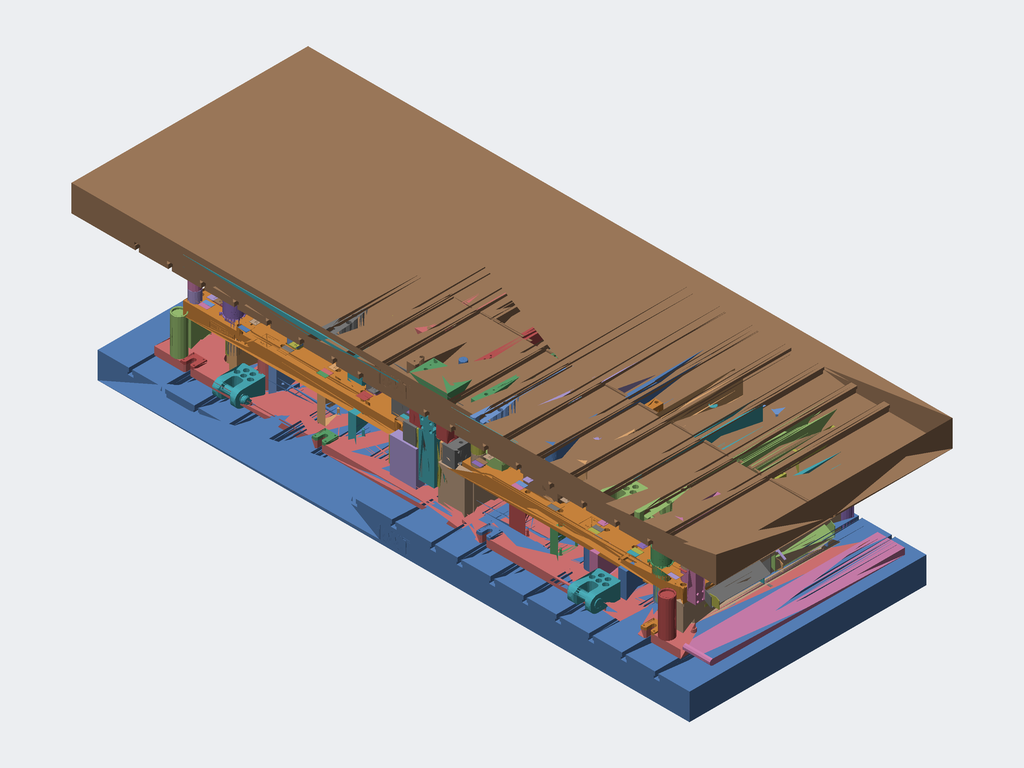Assembly | STEP file | 1269 different items | 1269 placed
Parts list (item | name | quantity | parent item | size | volume), first 346 of 1269 items:
1 | 008_id4090_x_t | x1 | in lll_x_t | 80 x 80 x 85 mm | 404567 mm3
2 | 008_id4094_x_t | x1 | in lll_x_t | 80 x 80 x 85 mm | 404567 mm3
3 | 008_id4098_x_t | x1 | in lll_x_t | 80 x 80 x 85 mm | 404567 mm3
4 | 008_id4122_x_t | x1 | in lll_x_t | 80 x 80 x 85 mm | 404311 mm3
5 | 008_id4126_x_t | x1 | in lll_x_t | 80 x 80 x 85 mm | 404567 mm3
6 | 008_id4130_x_t | x1 | in lll_x_t | 80 x 80 x 85 mm | 404311 mm3
7 | 014_id2546_x_t | x1 | in lll_x_t | 80 x 80 x 137.5 mm | 639951 mm3
8 | 014_id2550_x_t | x1 | in lll_x_t | 80 x 80 x 137.5 mm | 639951 mm3
9 | 014_id2554_x_t | x1 | in lll_x_t | 80 x 80 x 137.5 mm | 639951 mm3
10 | 014_id2558_x_t | x1 | in lll_x_t | 80 x 80 x 137.5 mm | 639951 mm3
11 | 014_id2562_x_t | x1 | in lll_x_t | 80 x 80 x 137.5 mm | 639951 mm3
12 | 014_id2842_x_t | x1 | in lll_x_t | 80 x 80 x 137.5 mm | 639951 mm3
13 | 103_id3510_x_t | x1 | in lll_x_t | 115 x 32.999 x 20 mm | 61100 mm3
14 | 180_id4502_x_t | x1 | in lll_x_t | 235 x 230 x 80 mm | 2542104 mm3
15 | 180_id4582_x_t | x1 | in lll_x_t | 565 x 500 x 35 mm | 7605579 mm3
16 | 1_id1746_x_t | x1 | in lll_x_t | 36 x 36 x 216 mm | 99455 mm3
17 | 1_id1750_x_t | x1 | in lll_x_t | 36 x 36 x 216 mm | 99455 mm3
18 | 1_id1758_x_t | x1 | in lll_x_t | 36 x 36 x 216 mm | 99455 mm3
19 | 1_id1798_x_t | x1 | in lll_x_t | 18 x 18 x 52 mm | 7011 mm3
20 | 1_id1802_x_t | x1 | in lll_x_t | 18 x 18 x 52 mm | 7011 mm3
21 | 1_id1806_x_t | x1 | in lll_x_t | 18 x 18 x 52 mm | 7011 mm3
22 | 1_id1814_x_t | x1 | in lll_x_t | 18 x 18 x 52 mm | 7011 mm3
23 | 1_id1822_x_t | x1 | in lll_x_t | 18 x 18 x 52 mm | 7011 mm3
24 | 1_id1826_x_t | x1 | in lll_x_t | 18 x 18 x 52 mm | 7011 mm3
25 | 1_id1834_x_t | x1 | in lll_x_t | 18 x 18 x 52 mm | 7011 mm3
26 | 1_id1846_x_t | x1 | in lll_x_t | 18 x 18 x 52 mm | 7011 mm3
27 | 1_id1850_x_t | x1 | in lll_x_t | 18 x 18 x 52 mm | 7011 mm3
28 | 1_id1862_x_t | x1 | in lll_x_t | 18 x 18 x 52 mm | 7011 mm3
29 | 1_id1866_x_t | x1 | in lll_x_t | 18 x 18 x 52 mm | 7011 mm3
30 | 1_id1870_x_t | x1 | in lll_x_t | 18 x 18 x 52 mm | 7011 mm3
31 | 1_id1882_x_t | x1 | in lll_x_t | 18 x 18 x 52 mm | 7011 mm3
32 | 1_id1886_x_t | x1 | in lll_x_t | 18 x 18 x 52 mm | 7011 mm3
33 | 1_id1890_x_t | x1 | in lll_x_t | 18 x 18 x 52 mm | 7011 mm3
34 | 1_id1894_x_t | x1 | in lll_x_t | 18 x 18 x 52 mm | 7011 mm3
35 | 1_id1898_x_t | x1 | in lll_x_t | 18 x 18 x 52 mm | 7011 mm3
36 | 1_id1902_x_t | x1 | in lll_x_t | 18 x 18 x 52 mm | 7011 mm3
37 | 1_id1910_x_t | x1 | in lll_x_t | 18 x 18 x 52 mm | 7011 mm3
38 | 1_id1914_x_t | x1 | in lll_x_t | 18 x 18 x 52 mm | 7011 mm3
39 | 1_id1922_x_t | x1 | in lll_x_t | 18 x 18 x 52 mm | 7011 mm3
40 | 1_id1930_x_t | x1 | in lll_x_t | 18 x 18 x 52 mm | 7011 mm3
41 | 1_id1934_x_t | x1 | in lll_x_t | 18 x 18 x 52 mm | 7011 mm3
42 | 1_id1942_x_t | x1 | in lll_x_t | 18 x 18 x 52 mm | 7011 mm3
43 | 1_id1950_x_t | x1 | in lll_x_t | 18 x 18 x 52 mm | 7011 mm3
44 | 1_id1954_x_t | x1 | in lll_x_t | 18 x 18 x 52 mm | 7011 mm3
45 | 1_id1962_x_t | x1 | in lll_x_t | 18 x 18 x 52 mm | 7011 mm3
46 | 1_id1970_x_t | x1 | in lll_x_t | 18 x 18 x 52 mm | 7011 mm3
47 | 1_id1974_x_t | x1 | in lll_x_t | 18 x 18 x 52 mm | 7011 mm3
48 | 1_id1982_x_t | x1 | in lll_x_t | 18 x 18 x 52 mm | 7011 mm3
49 | 1_id1990_x_t | x1 | in lll_x_t | 18 x 18 x 52 mm | 7011 mm3
50 | 1_id1994_x_t | x1 | in lll_x_t | 18 x 18 x 52 mm | 7011 mm3
51 | 1_id2002_x_t | x1 | in lll_x_t | 18 x 18 x 52 mm | 7011 mm3
52 | 1_id2010_x_t | x1 | in lll_x_t | 18 x 18 x 52 mm | 7011 mm3
53 | 1_id2014_x_t | x1 | in lll_x_t | 18 x 18 x 52 mm | 7011 mm3
54 | 1_id2022_x_t | x1 | in lll_x_t | 18 x 18 x 52 mm | 7011 mm3
55 | 1_id2030_x_t | x1 | in lll_x_t | 18 x 18 x 52 mm | 7011 mm3
56 | 1_id2034_x_t | x1 | in lll_x_t | 18 x 18 x 52 mm | 7011 mm3
57 | 1_id2042_x_t | x1 | in lll_x_t | 18 x 18 x 52 mm | 7011 mm3
58 | 1_id2050_x_t | x1 | in lll_x_t | 18 x 18 x 52 mm | 7011 mm3
59 | 1_id2054_x_t | x1 | in lll_x_t | 18 x 18 x 52 mm | 7011 mm3
60 | 1_id2062_x_t | x1 | in lll_x_t | 18 x 18 x 52 mm | 7011 mm3
61 | 1_id2066_x_t | x1 | in lll_x_t | 18 x 18 x 52 mm | 7011 mm3
62 | 1_id2070_x_t | x1 | in lll_x_t | 18 x 18 x 52 mm | 7011 mm3
63 | 1_id2074_x_t | x1 | in lll_x_t | 18 x 18 x 52 mm | 7011 mm3
64 | 1_id2086_x_t | x1 | in lll_x_t | 18 x 18 x 52 mm | 7011 mm3
65 | 1_id2090_x_t | x1 | in lll_x_t | 18 x 18 x 52 mm | 7011 mm3
66 | 1_id2094_x_t | x1 | in lll_x_t | 18 x 18 x 52 mm | 7011 mm3
67 | 1_id2114_x_t | x1 | in lll_x_t | 18 x 18 x 52 mm | 7011 mm3
68 | 1_id2118_x_t | x1 | in lll_x_t | 18 x 18 x 52 mm | 7011 mm3
69 | 1_id2122_x_t | x1 | in lll_x_t | 18 x 18 x 52 mm | 7011 mm3
70 | 1_id2126_x_t | x1 | in lll_x_t | 18 x 18 x 52 mm | 7011 mm3
71 | 1_id2130_x_t | x1 | in lll_x_t | 18 x 18 x 52 mm | 7011 mm3
72 | 1_id2134_x_t | x1 | in lll_x_t | 18 x 18 x 52 mm | 7011 mm3
73 | 1_id2138_x_t | x1 | in lll_x_t | 18 x 18 x 52 mm | 7011 mm3
74 | 1_id2142_x_t | x1 | in lll_x_t | 18 x 18 x 52 mm | 7011 mm3
75 | 1_id2310_x_t | x1 | in lll_x_t | 63.2 x 63.2 x 294 mm | 592651 mm3
76 | 1_id2330_x_t | x1 | in lll_x_t | 75.2 x 75.2 x 295 mm | 855529 mm3
77 | 1_id2338_x_t | x1 | in lll_x_t | 63.2 x 63.2 x 294 mm | 592651 mm3
78 | 1_id2346_x_t | x1 | in lll_x_t | 63.2 x 63.2 x 294 mm | 592651 mm3
79 | 1_id2358_x_t | x1 | in lll_x_t | 63.2 x 63.2 x 294 mm | 592651 mm3
80 | 1_id2362_x_t | x1 | in lll_x_t | 63.2 x 63.2 x 294 mm | 592651 mm3
81 | 1_id2366_x_t | x1 | in lll_x_t | 63.2 x 63.2 x 294 mm | 592651 mm3
82 | 1_id2370_x_t | x1 | in lll_x_t | 63.2 x 63.2 x 294 mm | 592651 mm3
83 | 1_id2374_x_t | x1 | in lll_x_t | 63.2 x 63.2 x 294 mm | 592651 mm3
84 | 1_id2378_x_t | x1 | in lll_x_t | 63.2 x 63.2 x 294 mm | 592651 mm3
85 | 1_id2382_x_t | x1 | in lll_x_t | 63.2 x 63.2 x 294 mm | 592651 mm3
86 | 1_id2386_x_t | x1 | in lll_x_t | 63.2 x 63.2 x 294 mm | 592651 mm3
87 | 1_id2390_x_t | x1 | in lll_x_t | 63.2 x 63.2 x 294 mm | 592651 mm3
88 | 1_id2394_x_t | x1 | in lll_x_t | 63.2 x 63.2 x 294 mm | 592651 mm3
89 | 1_id2398_x_t | x1 | in lll_x_t | 63.2 x 63.2 x 294 mm | 592651 mm3
90 | 1_id2402_x_t | x1 | in lll_x_t | 63.2 x 63.2 x 294 mm | 592651 mm3
91 | 1_id2406_x_t | x1 | in lll_x_t | 63.2 x 63.2 x 294 mm | 592651 mm3
92 | 1_id2410_x_t | x1 | in lll_x_t | 63.2 x 63.2 x 294 mm | 592651 mm3
93 | 1_id2414_x_t | x1 | in lll_x_t | 63.2 x 63.2 x 294 mm | 592651 mm3
94 | 1_id2418_x_t | x1 | in lll_x_t | 75.2 x 75.2 x 295 mm | 855529 mm3
95 | 1_id2422_x_t | x1 | in lll_x_t | 63.2 x 63.2 x 294 mm | 592651 mm3
96 | 1_id2426_x_t | x1 | in lll_x_t | 63.2 x 63.2 x 294 mm | 592651 mm3
97 | 1_id2430_x_t | x1 | in lll_x_t | 63.2 x 63.2 x 294 mm | 592651 mm3
98 | 1_id2434_x_t | x1 | in lll_x_t | 63.2 x 63.2 x 294 mm | 592651 mm3
99 | 1_id2438_x_t | x1 | in lll_x_t | 63.2 x 63.2 x 294 mm | 592651 mm3
100 | 1_id2442_x_t | x1 | in lll_x_t | 63.2 x 63.2 x 294 mm | 592651 mm3
101 | 1_id2446_x_t | x1 | in lll_x_t | 63.2 x 63.2 x 294 mm | 592651 mm3
102 | 1_id2450_x_t | x1 | in lll_x_t | 63.2 x 63.2 x 294 mm | 592651 mm3
103 | 1_id2454_x_t | x1 | in lll_x_t | 75.2 x 75.2 x 295 mm | 855529 mm3
104 | 1_id2458_x_t | x1 | in lll_x_t | 95.2 x 95.2 x 308 mm | 1486829 mm3
105 | 1_id2462_x_t | x1 | in lll_x_t | 95.2 x 95.2 x 308 mm | 1486829 mm3
106 | 1_id2482_x_t | x1 | in lll_x_t | 217 x 240 x 120 mm | 3421641 mm3
107 | 1_id2486_x_t | x1 | in lll_x_t | 217 x 240 x 120 mm | 3421641 mm3
108 | 1_id2518_x_t | x1 | in lll_x_t | 36 x 36 x 216 mm | 99455 mm3
109 | 1_id2522_x_t | x1 | in lll_x_t | 36 x 36 x 216 mm | 99455 mm3
110 | 1_id2526_x_t | x1 | in lll_x_t | 36 x 36 x 216 mm | 99455 mm3
111 | 1_id282_x_t | x1 | in lll_x_t | 21 x 21 x 118.2 mm | 17923 mm3
112 | 1_id286_x_t | x1 | in lll_x_t | 21 x 21 x 118.2 mm | 17923 mm3
113 | 1_id290_x_t | x1 | in lll_x_t | 43 x 39 x 118.2 mm | 84183 mm3
114 | 1_id294_x_t | x1 | in lll_x_t | 43 x 39 x 118.2 mm | 84183 mm3
115 | 1_id3518_x_t | x1 | in lll_x_t | 37 x 37 x 118.2 mm | 77419 mm3
116 | 1_id3530_x_t | x1 | in lll_x_t | 37 x 37 x 118.2 mm | 77419 mm3
117 | 1_id3546_x_t | x1 | in lll_x_t | 37 x 37 x 118.2 mm | 77419 mm3
118 | 1_id3566_x_t | x1 | in lll_x_t | 30 x 26 x 118.2 mm | 45235 mm3
119 | 1_id3570_x_t | x1 | in lll_x_t | 37 x 37 x 118.2 mm | 77419 mm3
120 | 1_id3590_x_t | x1 | in lll_x_t | 37 x 37 x 118.2 mm | 77419 mm3
121 | 1_id3618_x_t | x1 | in lll_x_t | 37 x 37 x 118.2 mm | 77419 mm3
122 | 1_id3630_x_t | x1 | in lll_x_t | 37 x 37 x 118.2 mm | 77419 mm3
123 | 1_id3642_x_t | x1 | in lll_x_t | 25 x 22.5 x 118.2 mm | 27347 mm3
124 | 1_id3650_x_t | x1 | in lll_x_t | 30 x 26 x 118.2 mm | 45235 mm3
125 | 1_id3662_x_t | x1 | in lll_x_t | 25 x 25 x 118.2 mm | 30521 mm3
126 | 1_id3670_x_t | x1 | in lll_x_t | 25 x 25 x 118.2 mm | 30521 mm3
127 | 1_id3686_x_t | x1 | in lll_x_t | 25 x 22.5 x 118.2 mm | 27347 mm3
128 | 1_id3690_x_t | x1 | in lll_x_t | 37 x 37 x 118.2 mm | 77419 mm3
129 | 1_id3750_x_t | x1 | in lll_x_t | 28 x 28 x 222 mm | 65272 mm3
130 | 1_id3758_x_t | x1 | in lll_x_t | 28 x 28 x 222 mm | 65272 mm3
131 | 1_id3922_x_t | x1 | in lll_x_t | 45.2 x 45.2 x 405 mm | 414792 mm3
132 | 1_id3926_x_t | x1 | in lll_x_t | 45.2 x 45.2 x 405 mm | 414792 mm3
133 | 1_id3930_x_t | x1 | in lll_x_t | 45.2 x 45.2 x 405 mm | 414792 mm3
134 | 1_id3934_x_t | x1 | in lll_x_t | 45.2 x 45.2 x 405 mm | 414792 mm3
135 | 1_id3938_x_t | x1 | in lll_x_t | 45.2 x 45.2 x 405 mm | 414792 mm3
136 | 1_id3942_x_t | x1 | in lll_x_t | 45.2 x 45.2 x 405 mm | 414792 mm3
137 | 1_id3946_x_t | x1 | in lll_x_t | 45.2 x 45.2 x 405 mm | 414792 mm3
138 | 1_id3950_x_t | x1 | in lll_x_t | 45.2 x 45.2 x 405 mm | 414792 mm3
139 | 1_id3954_x_t | x1 | in lll_x_t | 45.2 x 45.2 x 405 mm | 414792 mm3
140 | 1_id3958_x_t | x1 | in lll_x_t | 45.2 x 45.2 x 405 mm | 414792 mm3
141 | 1_id3962_x_t | x1 | in lll_x_t | 45.2 x 45.2 x 405 mm | 414792 mm3
142 | 1_id3966_x_t | x1 | in lll_x_t | 45.2 x 45.2 x 405 mm | 414792 mm3
143 | 1_id3970_x_t | x1 | in lll_x_t | 45.2 x 45.2 x 405 mm | 414792 mm3
144 | 1_id3974_x_t | x1 | in lll_x_t | 45.2 x 45.2 x 405 mm | 414792 mm3
145 | 1_id3978_x_t | x1 | in lll_x_t | 45.2 x 45.2 x 405 mm | 414792 mm3
146 | 1_id4158_x_t | x1 | in lll_x_t | 16 x 16 x 40 mm | 4057 mm3
147 | 1_id4170_x_t | x1 | in lll_x_t | 16 x 16 x 40 mm | 4057 mm3
148 | 1_id4174_x_t | x1 | in lll_x_t | 16 x 16 x 40 mm | 4057 mm3
149 | 1_id4178_x_t | x1 | in lll_x_t | 16 x 16 x 40 mm | 4057 mm3
150 | 1_id4182_x_t | x1 | in lll_x_t | 16 x 16 x 40 mm | 4057 mm3
151 | 1_id4402_x_t | x1 | in lll_x_t | 217 x 240 x 120 mm | 3421641 mm3
152 | 1_id4426_x_t | x1 | in lll_x_t | 36 x 36 x 236 mm | 108861 mm3
153 | 1_id4430_x_t | x1 | in lll_x_t | 36 x 36 x 236 mm | 108861 mm3
154 | 1_id4434_x_t | x1 | in lll_x_t | 36 x 36 x 236 mm | 108861 mm3
155 | 1_id4442_x_t | x1 | in lll_x_t | 36 x 36 x 236 mm | 108861 mm3
156 | 1_id4530_x_t | x1 | in lll_x_t | 38 x 37.821 x 35 mm | 25400 mm3
157 | 1_id4534_x_t | x1 | in lll_x_t | 32 x 32 x 35 mm | 19058 mm3
158 | 1_id4546_x_t | x1 | in lll_x_t | 32 x 32 x 35 mm | 19791 mm3
159 | 1_id4566_x_t | x1 | in lll_x_t | 38 x 36.5 x 35 mm | 27105 mm3
160 | 1_id4750_x_t | x1 | in lll_x_t | 36 x 36 x 236 mm | 108861 mm3
161 | 1_id4754_x_t | x1 | in lll_x_t | 36 x 36 x 236 mm | 108861 mm3
162 | 1_id4774_x_t | x1 | in lll_x_t | 36 x 36 x 236 mm | 108861 mm3
163 | 1_id4802_x_t | x1 | in lll_x_t | 36 x 36 x 236 mm | 108861 mm3
164 | 1_id4814_x_t | x1 | in lll_x_t | 36 x 36 x 236 mm | 108861 mm3
165 | 1_id4818_x_t | x1 | in lll_x_t | 36 x 36 x 236 mm | 108861 mm3
166 | 1_id4882_x_t | x1 | in lll_x_t | 36 x 36 x 236 mm | 108861 mm3
167 | 1_id4886_x_t | x1 | in lll_x_t | 36 x 36 x 236 mm | 108861 mm3
168 | 1_id4890_x_t | x1 | in lll_x_t | 36 x 36 x 236 mm | 108861 mm3
169 | 1_id4902_x_t | x1 | in lll_x_t | 36 x 36 x 236 mm | 108861 mm3
170 | 1_id870_x_t | x1 | in lll_x_t | 217 x 240 x 120 mm | 3421641 mm3
171 | 1_id874_x_t | x1 | in lll_x_t | 217 x 240 x 120 mm | 3421641 mm3
172 | 1_id878_x_t | x1 | in lll_x_t | 217 x 240 x 120 mm | 3421641 mm3
173 | 1_id882_x_t | x1 | in lll_x_t | 217 x 240 x 120 mm | 3421641 mm3
174 | 1_id886_x_t | x1 | in lll_x_t | 217 x 240 x 120 mm | 3421641 mm3
175 | APJAL13-100-P6.56_2_id106_x_t | x1 | in lll_x_t | 18 x 18 x 100 mm | 10594 mm3
176 | APJAL13-100-P6.56_2_id122_x_t | x1 | in lll_x_t | 18 x 18 x 100 mm | 10594 mm3
177 | K8D2-17C930-A-INS-01_id190_x_t | x1 | in lll_x_t | 305 x 286.849 x 101.505 mm | 137938 mm3
178 | K8D2-17C930-A-INS-01_id26_x_t | x1 | in lll_x_t | 305 x 286.849 x 101.505 mm | 137938 mm3
179 | K8D2-17C930-A-INS-01_id34_x_t | x1 | in lll_x_t | 305 x 286.849 x 101.505 mm | 137938 mm3
180 | K8D2-17C930-A-INS-01_id390_x_t | x1 | in lll_x_t | 305 x 286.849 x 101.505 mm | 137938 mm3
181 | K8D2-17C930-A-INS-01_id394_x_t | x1 | in lll_x_t | 305 x 286.849 x 101.505 mm | 137938 mm3
182 | K8D2-17C931-A-INS-01_id170_x_t | x1 | in lll_x_t | - | -
183 | K8D2-17C931-A-INS-01_id186_x_t | x1 | in lll_x_t | 305 x 288.457 x 93.294 mm | 168415 mm3
184 | K8D2-17C931-A-INS-01_id194_x_t | x1 | in lll_x_t | 305 x 286.852 x 101.506 mm | 138048 mm3
185 | K8D2-17C931-A-INS-01_id22_x_t | x1 | in lll_x_t | 305 x 286.852 x 101.506 mm | 138048 mm3
186 | K8D2-17C931-A-INS-01_id330_x_t | x1 | in lll_x_t | 305 x 288.457 x 93.294 mm | 168415 mm3
187 | K8D2-17C931-A-INS-01_id362_x_t | x1 | in lll_x_t | 305 x 286.852 x 101.506 mm | 138048 mm3
188 | K8D2-17C931-A-INS-01_id38_x_t | x1 | in lll_x_t | 305 x 286.852 x 101.506 mm | 138048 mm3
189 | K8D2-17C931-A-INS-01_id398_x_t | x1 | in lll_x_t | 305 x 286.852 x 101.506 mm | 138048 mm3
190 | K8D2-17C931-A-INS-01_id54_x_t | x1 | in lll_x_t | 305 x 288.457 x 93.298 mm | 168343 mm3
191 | lll_id1002_x_t | x1 | in lll_x_t | 40 x 5 x 2.5 mm | 497.027 mm3
192 | lll_id1006_x_t | x1 | in lll_x_t | 20 x 5 x 2.5 mm | 247.732 mm3
193 | lll_id1010_x_t | x1 | in lll_x_t | 68.033 x 31.95 x 1 mm | 2157 mm3
194 | lll_id1014_x_t | x1 | in lll_x_t | 68.033 x 31.95 x 1 mm | 2157 mm3
195 | lll_id1018_x_t | x1 | in lll_x_t | 68.033 x 31.95 x 1 mm | 2158 mm3
196 | lll_id1022_x_t | x1 | in lll_x_t | 68.033 x 31.95 x 1 mm | 2155 mm3
197 | lll_id1026_x_t | x1 | in lll_x_t | 68.033 x 31.95 x 1 mm | 2155 mm3
198 | lll_id102_x_t | x1 | in lll_x_t | 29 x 50 x 32 mm | 34441 mm3
199 | lll_id1030_x_t | x1 | in lll_x_t | 68.033 x 31.95 x 1 mm | 2157 mm3
200 | lll_id1034_x_t | x1 | in lll_x_t | 68.033 x 31.95 x 1 mm | 2157 mm3
201 | lll_id1038_x_t | x1 | in lll_x_t | 68.033 x 31.95 x 1 mm | 2157 mm3
202 | lll_id1042_x_t | x1 | in lll_x_t | 68.033 x 31.95 x 1 mm | 2157 mm3
203 | lll_id1046_x_t | x1 | in lll_x_t | 68.033 x 31.95 x 1 mm | 2157 mm3
204 | lll_id1050_x_t | x1 | in lll_x_t | 50 x 50 x 2 mm | 4932 mm3
205 | lll_id1054_x_t | x1 | in lll_x_t | 68.033 x 31.95 x 1 mm | 2157 mm3
206 | lll_id1058_x_t | x1 | in lll_x_t | 120 x 80 x 4 mm | 38260 mm3
207 | lll_id1062_x_t | x1 | in lll_x_t | 8.162 x 15.502 x 1 mm | 60.192 mm3
208 | lll_id1066_x_t | x1 | in lll_x_t | 11.813 x 15.95 x 1 mm | 65.616 mm3
209 | lll_id1070_x_t | x1 | in lll_x_t | 9.426 x 15.432 x 1 mm | 57.711 mm3
210 | lll_id1074_x_t | x1 | in lll_x_t | 8.049 x 15.752 x 1 mm | 54.602 mm3
211 | lll_id1078_x_t | x1 | in lll_x_t | 68.033 x 31.95 x 1 mm | 2174 mm3
212 | lll_id1082_x_t | x1 | in lll_x_t | 4.557 x 15.502 x 1 mm | 21.922 mm3
213 | lll_id1086_x_t | x1 | in lll_x_t | 1.938 x 1.285 x 2.5 mm | 3.455 mm3
214 | lll_id1090_x_t | x1 | in lll_x_t | 1.742 x 2.385 x 2.5 mm | 5.148 mm3
215 | lll_id1094_x_t | x1 | in lll_x_t | 2.571 x 2.384 x 2.5 mm | 9.133 mm3
216 | lll_id1098_x_t | x1 | in lll_x_t | 2.479 x 2.385 x 2.5 mm | 7.725 mm3
217 | lll_id10_x_t | x1 | in lll_x_t | 1050 x 805 x 35 mm | 22562559 mm3
218 | lll_id1102_x_t | x1 | in lll_x_t | 2.284 x 2.506 x 2.5 mm | 8.969 mm3
219 | lll_id1106_x_t | x1 | in lll_x_t | 2.9 x 2.384 x 2.5 mm | 9.219 mm3
220 | lll_id110_x_t | x1 | in lll_x_t | 260 x 104 x 32 mm | 608123 mm3
221 | lll_id1110_x_t | x1 | in lll_x_t | 20 x 10.473 x 2.5 mm | 50.145 mm3
222 | lll_id1114_x_t | x1 | in lll_x_t | 2.507 x 2.385 x 2.5 mm | 6.979 mm3
223 | lll_id1118_x_t | x1 | in lll_x_t | 2.599 x 2.384 x 2.5 mm | 9.059 mm3
224 | lll_id1122_x_t | x1 | in lll_x_t | 2.495 x 2.384 x 2.5 mm | 7.215 mm3
225 | lll_id1126_x_t | x1 | in lll_x_t | 1.938 x 1.285 x 2.5 mm | 3.454 mm3
226 | lll_id1130_x_t | x1 | in lll_x_t | 2.566 x 2.385 x 2.5 mm | 9.14 mm3
227 | lll_id1134_x_t | x1 | in lll_x_t | 13 x 13 x 2.5 mm | 49.087 mm3
228 | lll_id1138_x_t | x1 | in lll_x_t | 3.85 x 6 x 2.5 mm | 18.1 mm3
229 | lll_id1142_x_t | x1 | in lll_x_t | 20 x 5 x 2.5 mm | 247.732 mm3
230 | lll_id1146_x_t | x1 | in lll_x_t | 4.011 x 6 x 2.5 mm | 30.988 mm3
231 | lll_id114_x_t | x1 | in lll_x_t | 260 x 104 x 10 mm | 236864 mm3
232 | lll_id1150_x_t | x1 | in lll_x_t | 13 x 13 x 2.5 mm | 49.087 mm3
233 | lll_id1154_x_t | x1 | in lll_x_t | 2.566 x 2.385 x 2.5 mm | 9.126 mm3
234 | lll_id1158_x_t | x1 | in lll_x_t | 1.938 x 1.285 x 2.5 mm | 3.454 mm3
235 | lll_id1162_x_t | x1 | in lll_x_t | 2.495 x 2.384 x 2.5 mm | 7.215 mm3
236 | lll_id1166_x_t | x1 | in lll_x_t | 2.599 x 2.384 x 2.5 mm | 9.045 mm3
237 | lll_id1170_x_t | x1 | in lll_x_t | 2.507 x 2.385 x 2.5 mm | 6.979 mm3
238 | lll_id1174_x_t | x1 | in lll_x_t | 20 x 10.473 x 2.5 mm | 50.145 mm3
239 | lll_id1178_x_t | x1 | in lll_x_t | 2.9 x 2.384 x 2.5 mm | 9.21 mm3
240 | lll_id1182_x_t | x1 | in lll_x_t | 2.284 x 2.506 x 2.5 mm | 8.969 mm3
241 | lll_id1186_x_t | x1 | in lll_x_t | 2.479 x 2.385 x 2.5 mm | 7.725 mm3
242 | lll_id118_x_t | x1 | in lll_x_t | 50 x 29 x 32 mm | 32376 mm3
243 | lll_id1190_x_t | x1 | in lll_x_t | 2.571 x 2.384 x 2.5 mm | 9.13 mm3
244 | lll_id1194_x_t | x1 | in lll_x_t | 1.742 x 2.385 x 2.5 mm | 5.148 mm3
245 | lll_id1198_x_t | x1 | in lll_x_t | 1.938 x 1.285 x 2.5 mm | 3.455 mm3
246 | lll_id1202_x_t | x1 | in lll_x_t | 100 x 81 x 2.5 mm | 10066 mm3
247 | lll_id1206_x_t | x1 | in lll_x_t | 304.48 x 287.796 x 102.85 mm | 170516 mm3
248 | lll_id1210_x_t | x1 | in lll_x_t | 305 x 286.852 x 101.504 mm | 170099 mm3
249 | lll_id1214_x_t | x1 | in lll_x_t | 197 x 22 x 10 mm | 10197 mm3
250 | lll_id1218_x_t | x1 | in lll_x_t | 197 x 22 x 10 mm | 10197 mm3
251 | lll_id1222_x_t | x1 | in lll_x_t | 297 x 81 x 10 mm | 20263 mm3
252 | lll_id1226_x_t | x1 | in lll_x_t | 297 x 81 x 10 mm | 20263 mm3
253 | lll_id1230_x_t | x1 | in lll_x_t | 297 x 41 x 10 mm | 16253 mm3
254 | lll_id1234_x_t | x1 | in lll_x_t | 297 x 81.263 x 14.104 mm | 20343 mm3
255 | lll_id1238_x_t | x1 | in lll_x_t | 297 x 81 x 10 mm | 20263 mm3
256 | lll_id1242_x_t | x1 | in lll_x_t | 297 x 81 x 10 mm | 20263 mm3
257 | lll_id1246_x_t | x1 | in lll_x_t | 120.313 x 196.141 x 2.5 mm | 36784 mm3
258 | lll_id1250_x_t | x1 | in lll_x_t | 119.869 x 195.891 x 2.5 mm | 36599 mm3
259 | lll_id1254_x_t | x1 | in lll_x_t | 16.1 x 16.1 x 2.5 mm | 508.958 mm3
260 | lll_id1258_x_t | x1 | in lll_x_t | 16.1 x 16.1 x 2.5 mm | 508.958 mm3
261 | lll_id1262_x_t | x1 | in lll_x_t | 16.1 x 16.1 x 2.5 mm | 508.958 mm3
262 | lll_id1266_x_t | x1 | in lll_x_t | 28.07 x 28.07 x 2.5 mm | 1547 mm3
263 | lll_id126_x_t | x1 | in lll_x_t | 150 x 183 x 10 mm | 245447 mm3
264 | lll_id1270_x_t | x1 | in lll_x_t | 28.07 x 28.07 x 2.5 mm | 1547 mm3
265 | lll_id1274_x_t | x1 | in lll_x_t | 28.07 x 28.07 x 2.5 mm | 1547 mm3
266 | lll_id1278_x_t | x1 | in lll_x_t | 28.07 x 28.07 x 2.5 mm | 1547 mm3
267 | lll_id1282_x_t | x1 | in lll_x_t | 28.07 x 28.07 x 2.5 mm | 1547 mm3
268 | lll_id1286_x_t | x1 | in lll_x_t | 28.07 x 28.07 x 2.5 mm | 1547 mm3
269 | lll_id1290_x_t | x1 | in lll_x_t | 28.07 x 28.07 x 2.5 mm | 1547 mm3
270 | lll_id1294_x_t | x1 | in lll_x_t | 28.07 x 28.07 x 2.5 mm | 1547 mm3
271 | lll_id1298_x_t | x1 | in lll_x_t | 109.867 x 87.36 x 2.5 mm | 21961 mm3
272 | lll_id1302_x_t | x1 | in lll_x_t | 14.05 x 8.05 x 2.5 mm | 247.989 mm3
273 | lll_id1306_x_t | x1 | in lll_x_t | 50 x 50 x 2 mm | 4916 mm3
274 | lll_id130_x_t | x1 | in lll_x_t | 150 x 183 x 32 mm | 623652 mm3
275 | lll_id1310_x_t | x1 | in lll_x_t | 22.2 x 16.07 x 2.5 mm | 752.765 mm3
276 | lll_id1314_x_t | x1 | in lll_x_t | 16.07 x 16.07 x 2.5 mm | 507.063 mm3
277 | lll_id1318_x_t | x1 | in lll_x_t | 22.2 x 16.07 x 2.5 mm | 752.765 mm3
278 | lll_id1322_x_t | x1 | in lll_x_t | 16.07 x 16.07 x 2.5 mm | 507.063 mm3
279 | lll_id1326_x_t | x1 | in lll_x_t | 14.05 x 8.05 x 2.5 mm | 247.989 mm3
280 | lll_id1330_x_t | x1 | in lll_x_t | 16.07 x 16.07 x 2.5 mm | 507.063 mm3
281 | lll_id1334_x_t | x1 | in lll_x_t | 22.2 x 16.07 x 2.5 mm | 752.765 mm3
282 | lll_id1338_x_t | x1 | in lll_x_t | 68.033 x 31.95 x 1 mm | 2174 mm3
283 | lll_id1342_x_t | x1 | in lll_x_t | 8.049 x 15.752 x 1 mm | 54.602 mm3
284 | lll_id1346_x_t | x1 | in lll_x_t | 4.557 x 15.502 x 1 mm | 21.922 mm3
285 | lll_id134_x_t | x1 | in lll_x_t | 6.56 x 6.56 x 52.5 mm | 1774 mm3
286 | lll_id1350_x_t | x1 | in lll_x_t | 4.557 x 15.502 x 1 mm | 21.922 mm3
287 | lll_id1354_x_t | x1 | in lll_x_t | 9.426 x 15.432 x 1 mm | 57.711 mm3
288 | lll_id1358_x_t | x1 | in lll_x_t | 11.813 x 15.95 x 1 mm | 65.616 mm3
289 | lll_id1362_x_t | x1 | in lll_x_t | 68.033 x 31.95 x 1 mm | 2174 mm3
290 | lll_id1366_x_t | x1 | in lll_x_t | 8.049 x 15.752 x 1 mm | 54.602 mm3
291 | lll_id1370_x_t | x1 | in lll_x_t | 8.049 x 15.752 x 1 mm | 54.602 mm3
292 | lll_id1374_x_t | x1 | in lll_x_t | 4.557 x 15.502 x 1 mm | 21.922 mm3
293 | lll_id1378_x_t | x1 | in lll_x_t | 9.426 x 15.432 x 1 mm | 57.711 mm3
294 | lll_id1382_x_t | x1 | in lll_x_t | 11.813 x 15.95 x 1 mm | 65.616 mm3
295 | lll_id1386_x_t | x1 | in lll_x_t | 68.033 x 31.95 x 1 mm | 2174 mm3
296 | lll_id138_x_t | x1 | in lll_x_t | 6.56 x 6.56 x 52.5 mm | 1774 mm3
297 | lll_id1390_x_t | x1 | in lll_x_t | 8.049 x 15.752 x 1 mm | 54.602 mm3
298 | lll_id1394_x_t | x1 | in lll_x_t | 8.119 x 15.752 x 1 mm | 59.744 mm3
299 | lll_id1398_x_t | x1 | in lll_x_t | 8.049 x 15.752 x 1 mm | 54.602 mm3
300 | lll_id1402_x_t | x1 | in lll_x_t | 9.426 x 15.432 x 1 mm | 57.711 mm3
301 | lll_id1406_x_t | x1 | in lll_x_t | 11.813 x 15.95 x 1 mm | 65.616 mm3
302 | lll_id1410_x_t | x1 | in lll_x_t | 68.033 x 31.95 x 1 mm | 2174 mm3
303 | lll_id1414_x_t | x1 | in lll_x_t | 8.049 x 15.752 x 1 mm | 54.602 mm3
304 | lll_id1418_x_t | x1 | in lll_x_t | 8.132 x 15.752 x 1 mm | 58.959 mm3
305 | lll_id1422_x_t | x1 | in lll_x_t | 8.049 x 15.752 x 1 mm | 54.602 mm3
306 | lll_id1426_x_t | x1 | in lll_x_t | 9.426 x 15.432 x 1 mm | 57.711 mm3
307 | lll_id142_x_t | x1 | in lll_x_t | 44 x 90 x 38 mm | 119506 mm3
308 | lll_id1430_x_t | x1 | in lll_x_t | 11.813 x 15.95 x 1 mm | 65.616 mm3
309 | lll_id1434_x_t | x1 | in lll_x_t | 68.033 x 31.95 x 1 mm | 2174 mm3
310 | lll_id1438_x_t | x1 | in lll_x_t | 8.049 x 15.752 x 1 mm | 54.602 mm3
311 | lll_id1442_x_t | x1 | in lll_x_t | 7.993 x 15.234 x 1 mm | 34.068 mm3
312 | lll_id1446_x_t | x1 | in lll_x_t | 8.049 x 15.752 x 1 mm | 54.602 mm3
313 | lll_id1450_x_t | x1 | in lll_x_t | 9.426 x 15.432 x 1 mm | 57.711 mm3
314 | lll_id1454_x_t | x1 | in lll_x_t | 11.813 x 15.95 x 1 mm | 65.616 mm3
315 | lll_id1458_x_t | x1 | in lll_x_t | 68.033 x 31.95 x 1 mm | 2174 mm3
316 | lll_id1462_x_t | x1 | in lll_x_t | 8.049 x 15.752 x 1 mm | 54.602 mm3
317 | lll_id1466_x_t | x1 | in lll_x_t | 8.148 x 15.751 x 1 mm | 62.119 mm3
318 | lll_id146_x_t | x1 | in lll_x_t | 16 x 16 x 28 mm | 4560 mm3
319 | lll_id1470_x_t | x1 | in lll_x_t | 8.049 x 15.752 x 1 mm | 54.602 mm3
320 | lll_id1474_x_t | x1 | in lll_x_t | 9.426 x 15.432 x 1 mm | 57.711 mm3
321 | lll_id1478_x_t | x1 | in lll_x_t | 11.813 x 15.95 x 1 mm | 65.616 mm3
322 | lll_id1482_x_t | x1 | in lll_x_t | 68.033 x 31.95 x 1 mm | 2174 mm3
323 | lll_id1486_x_t | x1 | in lll_x_t | 8.049 x 15.752 x 1 mm | 54.602 mm3
324 | lll_id1490_x_t | x1 | in lll_x_t | 8.189 x 15.465 x 1 mm | 45.656 mm3
325 | lll_id1494_x_t | x1 | in lll_x_t | 8.049 x 15.752 x 1 mm | 54.602 mm3
326 | lll_id1498_x_t | x1 | in lll_x_t | 9.426 x 15.432 x 1 mm | 57.711 mm3
327 | lll_id14_x_t | x1 | in lll_x_t | 815 x 730 x 50 mm | 21862364 mm3
328 | lll_id1502_x_t | x1 | in lll_x_t | 11.813 x 15.95 x 1 mm | 65.616 mm3
329 | lll_id1506_x_t | x1 | in lll_x_t | 68.033 x 31.95 x 1 mm | 2174 mm3
330 | lll_id150_x_t | x1 | in lll_x_t | 125 x 170 x 38 mm | 581268 mm3
331 | lll_id1510_x_t | x1 | in lll_x_t | 8.049 x 15.752 x 1 mm | 54.602 mm3
332 | lll_id1514_x_t | x1 | in lll_x_t | 8.538 x 15.434 x 1 mm | 41.057 mm3
333 | lll_id1518_x_t | x1 | in lll_x_t | 8.049 x 15.752 x 1 mm | 54.602 mm3
334 | lll_id1522_x_t | x1 | in lll_x_t | 9.426 x 15.432 x 1 mm | 57.711 mm3
335 | lll_id1526_x_t | x1 | in lll_x_t | 11.813 x 15.95 x 1 mm | 65.616 mm3
336 | lll_id1530_x_t | x1 | in lll_x_t | 68.033 x 31.969 x 1 mm | 2175 mm3
337 | lll_id1534_x_t | x1 | in lll_x_t | 8.049 x 15.752 x 1 mm | 54.602 mm3
338 | lll_id1538_x_t | x1 | in lll_x_t | 8.074 x 15.771 x 1 mm | 33.504 mm3
339 | lll_id1542_x_t | x1 | in lll_x_t | 8.049 x 15.752 x 1 mm | 54.602 mm3
340 | lll_id1546_x_t | x1 | in lll_x_t | 9.426 x 15.432 x 1 mm | 57.711 mm3
341 | lll_id154_x_t | x1 | in lll_x_t | 6.56 x 6.56 x 52.5 mm | 1774 mm3
342 | lll_id1550_x_t | x1 | in lll_x_t | 11.813 x 15.95 x 1 mm | 65.616 mm3
343 | lll_id1554_x_t | x1 | in lll_x_t | 68.033 x 31.95 x 1 mm | 2174 mm3
344 | lll_id1558_x_t | x1 | in lll_x_t | 8.049 x 15.752 x 1 mm | 54.602 mm3
345 | lll_id1562_x_t | x1 | in lll_x_t | 8.162 x 15.502 x 1 mm | 60.192 mm3
346 | lll_id1566_x_t | x1 | in lll_x_t | 8.049 x 15.752 x 1 mm | 54.602 mm3